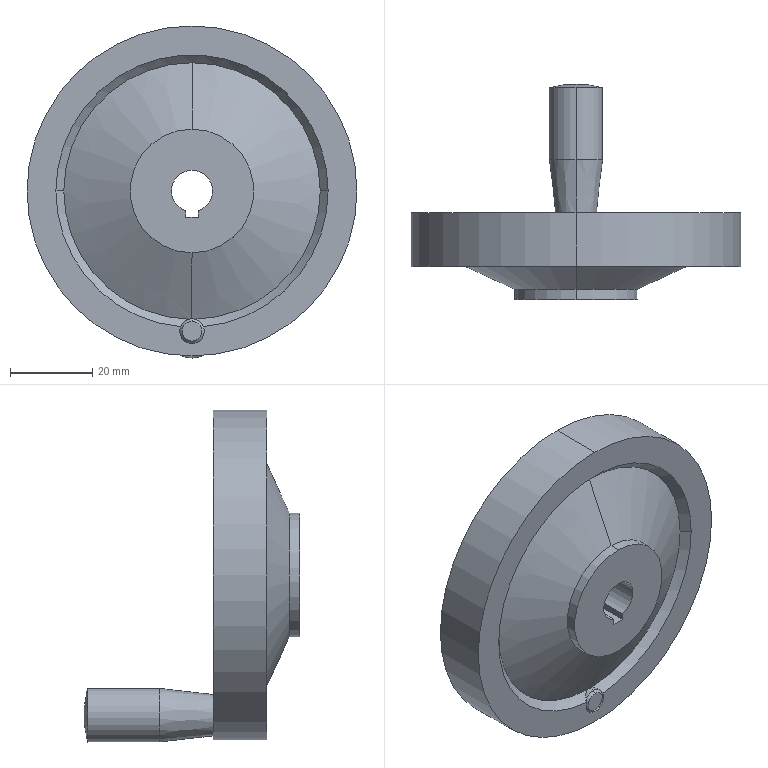Part | SolidWorks | features BaseBody 1 | 1 solid | 35 faces | box 80 x 52.448 x 80.5 mm | volume 63637 mm3 | cylinder 15 | cone 11 | plane 8 | spline 1 | commonest cylinder face diameters 30 x4 6 x3 10 x2 13 x2 56 x2 80 x2
STEP:
#1=CARTESIAN_POINT('',(0.,8.,40.));
#2=VERTEX_POINT('',#1);
#3=CARTESIAN_POINT('',(0.,8.,-40.));
#4=VERTEX_POINT('',#3);
#5=CARTESIAN_POINT('',(0.,8.,0.));
#6=DIRECTION('',(0.,1.,0.));
#7=DIRECTION('',(0.,0.,1.));
#8=AXIS2_PLACEMENT_3D('',#5,#6,#7);
#9=CIRCLE('',#8,40.);
#10=EDGE_CURVE('',#2,#4,#9,.T.);
#11=ORIENTED_EDGE('',*,*,#10,.T.);
#12=CARTESIAN_POINT('',(0.,21.,-40.));
#13=VERTEX_POINT('',#12);
#14=CARTESIAN_POINT('',(0.,-50.,-40.));
#15=DIRECTION('',(0.,1.,0.));
#16=VECTOR('',#15,1000.);
#17=LINE('',#14,#16);
#18=EDGE_CURVE('',#4,#13,#17,.T.);
#19=ORIENTED_EDGE('',*,*,#18,.T.);
#20=CARTESIAN_POINT('',(0.,21.,40.));
#21=VERTEX_POINT('',#20);
#22=CARTESIAN_POINT('',(0.,21.,0.));
#23=DIRECTION('',(0.,-1.,0.));
#24=DIRECTION('',(0.,0.,1.));
#25=AXIS2_PLACEMENT_3D('',#22,#23,#24);
#26=CIRCLE('',#25,40.);
#27=EDGE_CURVE('',#13,#21,#26,.T.);
#28=ORIENTED_EDGE('',*,*,#27,.T.);
#29=CARTESIAN_POINT('',(0.,-50.,40.));
#30=DIRECTION('',(0.,1.,0.));
#31=VECTOR('',#30,1000.);
#32=LINE('',#29,#31);
#33=EDGE_CURVE('',#2,#21,#32,.T.);
#34=ORIENTED_EDGE('',*,*,#33,.F.);
#35=EDGE_LOOP('',(#11,#19,#28,#34));
#36=FACE_OUTER_BOUND('',#35,.T.);
#37=CARTESIAN_POINT('',(0.,-50.,0.));
#38=DIRECTION('',(0.,1.,0.));
#39=DIRECTION('',(0.,0.,1.));
#40=AXIS2_PLACEMENT_3D('',#37,#38,#39);
#41=CYLINDRICAL_SURFACE('',#40,40.);
#42=ADVANCED_FACE('',(#36),#41,.T.);
#43=CARTESIAN_POINT('',(-31.09,9.91,0.));
#44=VERTEX_POINT('',#43);
#45=CARTESIAN_POINT('',(-0.6977,9.91,-31.082));
#46=VERTEX_POINT('',#45);
#47=CARTESIAN_POINT('',(0.,9.91,0.));
#48=DIRECTION('',(0.,-1.,0.));
#49=DIRECTION('',(0.,0.,-1.));
#50=AXIS2_PLACEMENT_3D('',#47,#48,#49);
#51=CIRCLE('',#50,31.09);
#52=EDGE_CURVE('',#44,#46,#51,.T.);
#53=ORIENTED_EDGE('',*,*,#52,.F.);
#54=CARTESIAN_POINT('',(-33.,8.,0.));
#55=VERTEX_POINT('',#54);
#56=CARTESIAN_POINT('',(-33.,8.,0.));
#57=DIRECTION('',(-0.7071,-0.7071,0.));
#58=VECTOR('',#57,1000.);
#59=LINE('',#56,#58);
#60=EDGE_CURVE('',#44,#55,#59,.T.);
#61=ORIENTED_EDGE('',*,*,#60,.T.);
#62=CARTESIAN_POINT('',(-2.784,8.,-32.882));
#63=VERTEX_POINT('',#62);
#64=CARTESIAN_POINT('',(0.,8.,0.));
#65=DIRECTION('',(0.,1.,0.));
#66=DIRECTION('',(1.,0.,0.));
#67=AXIS2_PLACEMENT_3D('',#64,#65,#66);
#68=CIRCLE('',#67,33.);
#69=EDGE_CURVE('',#63,#55,#68,.T.);
#70=ORIENTED_EDGE('',*,*,#69,.F.);
#71=CARTESIAN_POINT('',(-2.5,8.561,-32.342));
#72=VERTEX_POINT('',#71);
#73=CARTESIAN_POINT('',(-2.784,8.,-32.882));
#74=CARTESIAN_POINT('',(-2.709,8.192,-32.696));
#75=CARTESIAN_POINT('',(-2.616,8.379,-32.516));
#76=CARTESIAN_POINT('',(-2.5,8.561,-32.342));
#77=B_SPLINE_CURVE_WITH_KNOTS('',3,(#73,#74,#75,#76),.UNSPECIFIED.,.F.,.F.,(4,4),(0.,0.0008292),.UNSPECIFIED.);
#78=EDGE_CURVE('',#63,#72,#77,.T.);
#79=ORIENTED_EDGE('',*,*,#78,.T.);
#80=CARTESIAN_POINT('',(-0.6977,9.91,-31.082));
#81=CARTESIAN_POINT('',(-0.9084,9.855,-31.133));
#82=CARTESIAN_POINT('',(-1.102,9.778,-31.203));
#83=CARTESIAN_POINT('',(-1.463,9.593,-31.373));
#84=CARTESIAN_POINT('',(-1.63,9.483,-31.475));
#85=CARTESIAN_POINT('',(-2.078,9.129,-31.805));
#86=CARTESIAN_POINT('',(-2.315,8.853,-32.063));
#87=CARTESIAN_POINT('',(-2.5,8.561,-32.342));
#88=B_SPLINE_CURVE_WITH_KNOTS('',3,(#80,#81,#82,#83,#84,#85,#86,#87),.UNSPECIFIED.,.F.,.F.,(4,2,2,4),(0.,0.0006578,0.001316,0.002631),.UNSPECIFIED.);
#89=EDGE_CURVE('',#46,#72,#88,.T.);
#90=ORIENTED_EDGE('',*,*,#89,.F.);
#91=EDGE_LOOP('',(#53,#61,#70,#79,#90));
#92=FACE_OUTER_BOUND('',#91,.T.);
#93=CARTESIAN_POINT('',(0.,8.,0.));
#94=DIRECTION('',(0.,-1.,0.));
#95=DIRECTION('',(1.,0.,0.));
#96=AXIS2_PLACEMENT_3D('',#93,#94,#95);
#97=CONICAL_SURFACE('',#96,33.,0.7854);
#98=ADVANCED_FACE('',(#92),#97,.F.);
#99=ORIENTED_EDGE('',*,*,#60,.F.);
#100=CARTESIAN_POINT('',(0.,9.91,31.09));
#101=VERTEX_POINT('',#100);
#102=CARTESIAN_POINT('',(0.,9.91,0.));
#103=DIRECTION('',(0.,-1.,0.));
#104=DIRECTION('',(0.,0.,-1.));
#105=AXIS2_PLACEMENT_3D('',#102,#103,#104);
#106=CIRCLE('',#105,31.09);
#107=EDGE_CURVE('',#101,#44,#106,.T.);
#108=ORIENTED_EDGE('',*,*,#107,.F.);
#109=CARTESIAN_POINT('',(31.09,9.91,0.));
#110=VERTEX_POINT('',#109);
#111=CARTESIAN_POINT('',(0.,9.91,0.));
#112=DIRECTION('',(0.,-1.,0.));
#113=DIRECTION('',(0.,0.,-1.));
#114=AXIS2_PLACEMENT_3D('',#111,#112,#113);
#115=CIRCLE('',#114,31.09);
#116=EDGE_CURVE('',#110,#101,#115,.T.);
#117=ORIENTED_EDGE('',*,*,#116,.F.);
#118=CARTESIAN_POINT('',(33.,8.,0.));
#119=VERTEX_POINT('',#118);
#120=CARTESIAN_POINT('',(33.,8.,0.));
#121=DIRECTION('',(0.7071,-0.7071,0.));
#122=VECTOR('',#121,1000.);
#123=LINE('',#120,#122);
#124=EDGE_CURVE('',#110,#119,#123,.T.);
#125=ORIENTED_EDGE('',*,*,#124,.T.);
#126=CARTESIAN_POINT('',(0.,8.,0.));
#127=DIRECTION('',(0.,1.,0.));
#128=DIRECTION('',(1.,0.,0.));
#129=AXIS2_PLACEMENT_3D('',#126,#127,#128);
#130=CIRCLE('',#129,33.);
#131=EDGE_CURVE('',#55,#119,#130,.T.);
#132=ORIENTED_EDGE('',*,*,#131,.F.);
#133=EDGE_LOOP('',(#99,#108,#117,#125,#132));
#134=FACE_OUTER_BOUND('',#133,.T.);
#135=CARTESIAN_POINT('',(0.,8.,0.));
#136=DIRECTION('',(0.,-1.,0.));
#137=DIRECTION('',(1.,0.,0.));
#138=AXIS2_PLACEMENT_3D('',#135,#136,#137);
#139=CONICAL_SURFACE('',#138,33.,0.7854);
#140=ADVANCED_FACE('',(#134),#139,.F.);
#141=CARTESIAN_POINT('',(0.,21.,-39.006));
#142=VERTEX_POINT('',#141);
#143=CARTESIAN_POINT('',(0.,21.,-28.994));
#144=VERTEX_POINT('',#143);
#145=CARTESIAN_POINT('',(0.,21.,-34.));
#146=DIRECTION('',(0.,-1.,0.));
#147=DIRECTION('',(0.,0.,1.));
#148=AXIS2_PLACEMENT_3D('',#145,#146,#147);
#149=CIRCLE('',#148,5.006);
#150=EDGE_CURVE('',#142,#144,#149,.T.);
#151=ORIENTED_EDGE('',*,*,#150,.F.);
#152=CARTESIAN_POINT('',(0.,33.948,-40.5));
#153=VERTEX_POINT('',#152);
#154=CARTESIAN_POINT('',(0.,33.948,-40.5));
#155=DIRECTION('',(0.,0.9934,-0.1146));
#156=VECTOR('',#155,1000.);
#157=LINE('',#154,#156);
#158=EDGE_CURVE('',#142,#153,#157,.T.);
#159=ORIENTED_EDGE('',*,*,#158,.T.);
#160=CARTESIAN_POINT('',(0.,33.948,-27.5));
#161=VERTEX_POINT('',#160);
#162=CARTESIAN_POINT('',(0.,33.948,-34.));
#163=DIRECTION('',(0.,-1.,0.));
#164=DIRECTION('',(0.,0.,1.));
#165=AXIS2_PLACEMENT_3D('',#162,#163,#164);
#166=CIRCLE('',#165,6.5);
#167=EDGE_CURVE('',#153,#161,#166,.T.);
#168=ORIENTED_EDGE('',*,*,#167,.T.);
#169=CARTESIAN_POINT('',(0.,33.948,-27.5));
#170=DIRECTION('',(0.,0.9934,0.1146));
#171=VECTOR('',#170,1000.);
#172=LINE('',#169,#171);
#173=EDGE_CURVE('',#144,#161,#172,.T.);
#174=ORIENTED_EDGE('',*,*,#173,.F.);
#175=EDGE_LOOP('',(#151,#159,#168,#174));
#176=FACE_OUTER_BOUND('',#175,.T.);
#177=CARTESIAN_POINT('',(0.,33.948,-34.));
#178=DIRECTION('',(0.,1.,0.));
#179=DIRECTION('',(0.,0.,1.));
#180=AXIS2_PLACEMENT_3D('',#177,#178,#179);
#181=CONICAL_SURFACE('',#180,6.5,0.1149);
#182=ADVANCED_FACE('',(#176),#181,.T.);
#183=CARTESIAN_POINT('',(0.,17.75,-28.));
#184=VERTEX_POINT('',#183);
#185=CARTESIAN_POINT('',(0.,17.75,28.));
#186=VERTEX_POINT('',#185);
#187=CARTESIAN_POINT('',(0.,17.75,0.));
#188=DIRECTION('',(0.,1.,0.));
#189=DIRECTION('',(0.,0.,1.));
#190=AXIS2_PLACEMENT_3D('',#187,#188,#189);
#191=CIRCLE('',#190,28.);
#192=EDGE_CURVE('',#184,#186,#191,.T.);
#193=ORIENTED_EDGE('',*,*,#192,.F.);
#194=CARTESIAN_POINT('',(0.,21.,-28.));
#195=VERTEX_POINT('',#194);
#196=CARTESIAN_POINT('',(0.,-50.,-28.));
#197=DIRECTION('',(0.,1.,0.));
#198=VECTOR('',#197,1000.);
#199=LINE('',#196,#198);
#200=EDGE_CURVE('',#184,#195,#199,.T.);
#201=ORIENTED_EDGE('',*,*,#200,.T.);
#202=CARTESIAN_POINT('',(0.,21.,28.));
#203=VERTEX_POINT('',#202);
#204=CARTESIAN_POINT('',(0.,21.,0.));
#205=DIRECTION('',(0.,-1.,0.));
#206=DIRECTION('',(0.,0.,1.));
#207=AXIS2_PLACEMENT_3D('',#204,#205,#206);
#208=CIRCLE('',#207,28.);
#209=EDGE_CURVE('',#203,#195,#208,.T.);
#210=ORIENTED_EDGE('',*,*,#209,.F.);
#211=CARTESIAN_POINT('',(0.,-50.,28.));
#212=DIRECTION('',(0.,1.,0.));
#213=VECTOR('',#212,1000.);
#214=LINE('',#211,#213);
#215=EDGE_CURVE('',#186,#203,#214,.T.);
#216=ORIENTED_EDGE('',*,*,#215,.F.);
#217=EDGE_LOOP('',(#193,#201,#210,#216));
#218=FACE_OUTER_BOUND('',#217,.T.);
#219=CARTESIAN_POINT('',(0.,-50.,0.));
#220=DIRECTION('',(0.,1.,0.));
#221=DIRECTION('',(0.,0.,1.));
#222=AXIS2_PLACEMENT_3D('',#219,#220,#221);
#223=CYLINDRICAL_SURFACE('',#222,28.);
#224=ADVANCED_FACE('',(#218),#223,.F.);
#225=CARTESIAN_POINT('',(0.,7.948,-31.613));
#226=VERTEX_POINT('',#225);
#227=CARTESIAN_POINT('',(0.,7.948,-36.387));
#228=VERTEX_POINT('',#227);
#229=CARTESIAN_POINT('',(0.,7.948,-34.));
#230=DIRECTION('',(0.,1.,0.));
#231=DIRECTION('',(0.,0.,1.));
#232=AXIS2_PLACEMENT_3D('',#229,#230,#231);
#233=CIRCLE('',#232,2.387);
#234=EDGE_CURVE('',#226,#228,#233,.T.);
#235=ORIENTED_EDGE('',*,*,#234,.T.);
#236=CARTESIAN_POINT('',(0.,8.561,-37.));
#237=VERTEX_POINT('',#236);
#238=CARTESIAN_POINT('',(0.,8.561,-37.));
#239=DIRECTION('',(0.,0.7071,-0.7071));
#240=VECTOR('',#239,1000.);
#241=LINE('',#238,#240);
#242=EDGE_CURVE('',#228,#237,#241,.T.);
#243=ORIENTED_EDGE('',*,*,#242,.T.);
#244=CARTESIAN_POINT('',(2.5,8.561,-32.342));
#245=VERTEX_POINT('',#244);
#246=CARTESIAN_POINT('',(0.,8.561,-34.));
#247=DIRECTION('',(0.,-1.,0.));
#248=DIRECTION('',(0.,0.,1.));
#249=AXIS2_PLACEMENT_3D('',#246,#247,#248);
#250=CIRCLE('',#249,3.);
#251=EDGE_CURVE('',#237,#245,#250,.T.);
#252=ORIENTED_EDGE('',*,*,#251,.T.);
#253=CARTESIAN_POINT('',(0.,8.561,-31.));
#254=VERTEX_POINT('',#253);
#255=CARTESIAN_POINT('',(0.,8.561,-34.));
#256=DIRECTION('',(0.,-1.,0.));
#257=DIRECTION('',(0.,0.,1.));
#258=AXIS2_PLACEMENT_3D('',#255,#256,#257);
#259=CIRCLE('',#258,3.);
#260=EDGE_CURVE('',#245,#254,#259,.T.);
#261=ORIENTED_EDGE('',*,*,#260,.T.);
#262=CARTESIAN_POINT('',(0.,8.561,-31.));
#263=DIRECTION('',(0.,0.7071,0.7071));
#264=VECTOR('',#263,1000.);
#265=LINE('',#262,#264);
#266=EDGE_CURVE('',#226,#254,#265,.T.);
#267=ORIENTED_EDGE('',*,*,#266,.F.);
#268=EDGE_LOOP('',(#235,#243,#252,#261,#267));
#269=FACE_OUTER_BOUND('',#268,.T.);
#270=CARTESIAN_POINT('',(0.,8.561,-34.));
#271=DIRECTION('',(0.,1.,0.));
#272=DIRECTION('',(0.,0.,1.));
#273=AXIS2_PLACEMENT_3D('',#270,#271,#272);
#274=CONICAL_SURFACE('',#273,3.,0.7854);
#275=ADVANCED_FACE('',(#269),#274,.T.);
#276=CARTESIAN_POINT('',(0.,8.561,-34.));
#277=DIRECTION('',(0.,-1.,0.));
#278=DIRECTION('',(0.,0.,1.));
#279=AXIS2_PLACEMENT_3D('',#276,#277,#278);
#280=CIRCLE('',#279,3.);
#281=EDGE_CURVE('',#254,#72,#280,.T.);
#282=ORIENTED_EDGE('',*,*,#281,.F.);
#283=CARTESIAN_POINT('',(0.,9.868,-31.));
#284=VERTEX_POINT('',#283);
#285=CARTESIAN_POINT('',(0.,-50.052,-31.));
#286=DIRECTION('',(0.,1.,0.));
#287=VECTOR('',#286,1000.);
#288=LINE('',#285,#287);
#289=EDGE_CURVE('',#254,#284,#288,.T.);
#290=ORIENTED_EDGE('',*,*,#289,.T.);
#291=CARTESIAN_POINT('',(0.,9.868,-31.));
#292=CARTESIAN_POINT('',(-0.2338,9.868,-31.));
#293=CARTESIAN_POINT('',(-0.4696,9.882,-31.028));
#294=CARTESIAN_POINT('',(-0.6977,9.91,-31.082));
#295=B_SPLINE_CURVE_WITH_KNOTS('',3,(#291,#292,#293,#294),.UNSPECIFIED.,.F.,.F.,(4,4),(0.0007033,0.001401),.UNSPECIFIED.);
#296=EDGE_CURVE('',#284,#46,#295,.T.);
#297=ORIENTED_EDGE('',*,*,#296,.T.);
#298=ORIENTED_EDGE('',*,*,#89,.T.);
#299=EDGE_LOOP('',(#282,#290,#297,#298));
#300=FACE_OUTER_BOUND('',#299,.T.);
#301=CARTESIAN_POINT('',(0.,-50.052,-34.));
#302=DIRECTION('',(0.,1.,0.));
#303=DIRECTION('',(0.,0.,1.));
#304=AXIS2_PLACEMENT_3D('',#301,#302,#303);
#305=CYLINDRICAL_SURFACE('',#304,3.);
#306=ADVANCED_FACE('',(#300),#305,.T.);
#307=CARTESIAN_POINT('',(0.,2.5,15.));
#308=VERTEX_POINT('',#307);
#309=CARTESIAN_POINT('',(0.,2.5,-15.));
#310=VERTEX_POINT('',#309);
#311=CARTESIAN_POINT('',(0.,2.5,0.));
#312=DIRECTION('',(0.,1.,0.));
#313=DIRECTION('',(0.,0.,1.));
#314=AXIS2_PLACEMENT_3D('',#311,#312,#313);
#315=CIRCLE('',#314,15.);
#316=EDGE_CURVE('',#308,#310,#315,.T.);
#317=ORIENTED_EDGE('',*,*,#316,.T.);
#318=CARTESIAN_POINT('',(0.,9.91,-31.09));
#319=DIRECTION('',(0.,0.4183,-0.9083));
#320=VECTOR('',#319,1000.);
#321=LINE('',#318,#320);
#322=EDGE_CURVE('',#310,#284,#321,.T.);
#323=ORIENTED_EDGE('',*,*,#322,.T.);
#324=CARTESIAN_POINT('',(0.6977,9.91,-31.082));
#325=VERTEX_POINT('',#324);
#326=CARTESIAN_POINT('',(0.6977,9.91,-31.082));
#327=CARTESIAN_POINT('',(0.468,9.882,-31.027));
#328=CARTESIAN_POINT('',(0.2354,9.868,-31.));
#329=CARTESIAN_POINT('',(0.,9.868,-31.));
#330=B_SPLINE_CURVE_WITH_KNOTS('',3,(#326,#327,#328,#329),.UNSPECIFIED.,.F.,.F.,(4,4),(0.,0.0007033),.UNSPECIFIED.);
#331=EDGE_CURVE('',#325,#284,#330,.T.);
#332=ORIENTED_EDGE('',*,*,#331,.F.);
#333=CARTESIAN_POINT('',(0.,9.91,0.));
#334=DIRECTION('',(0.,-1.,0.));
#335=DIRECTION('',(0.,0.,-1.));
#336=AXIS2_PLACEMENT_3D('',#333,#334,#335);
#337=CIRCLE('',#336,31.09);
#338=EDGE_CURVE('',#325,#110,#337,.T.);
#339=ORIENTED_EDGE('',*,*,#338,.T.);
#340=ORIENTED_EDGE('',*,*,#116,.T.);
#341=CARTESIAN_POINT('',(0.,9.91,31.09));
#342=DIRECTION('',(0.,0.4183,0.9083));
#343=VECTOR('',#342,1000.);
#344=LINE('',#341,#343);
#345=EDGE_CURVE('',#308,#101,#344,.T.);
#346=ORIENTED_EDGE('',*,*,#345,.F.);
#347=EDGE_LOOP('',(#317,#323,#332,#339,#340,#346));
#348=FACE_OUTER_BOUND('',#347,.T.);
#349=CARTESIAN_POINT('',(0.,9.91,0.));
#350=DIRECTION('',(0.,1.,0.));
#351=DIRECTION('',(0.,0.,1.));
#352=AXIS2_PLACEMENT_3D('',#349,#350,#351);
#353=CONICAL_SURFACE('',#352,31.09,1.139);
#354=ADVANCED_FACE('',(#348),#353,.T.);
#355=ORIENTED_EDGE('',*,*,#167,.F.);
#356=CARTESIAN_POINT('',(0.,51.448,-40.5));
#357=VERTEX_POINT('',#356);
#358=CARTESIAN_POINT('',(0.,-50.052,-40.5));
#359=DIRECTION('',(0.,1.,0.));
#360=VECTOR('',#359,1000.);
#361=LINE('',#358,#360);
#362=EDGE_CURVE('',#153,#357,#361,.T.);
#363=ORIENTED_EDGE('',*,*,#362,.T.);
#364=CARTESIAN_POINT('',(0.,51.448,-27.5));
#365=VERTEX_POINT('',#364);
#366=CARTESIAN_POINT('',(0.,51.448,-34.));
#367=DIRECTION('',(0.,-1.,0.));
#368=DIRECTION('',(0.,0.,1.));
#369=AXIS2_PLACEMENT_3D('',#366,#367,#368);
#370=CIRCLE('',#369,6.5);
#371=EDGE_CURVE('',#357,#365,#370,.T.);
#372=ORIENTED_EDGE('',*,*,#371,.T.);
#373=CARTESIAN_POINT('',(0.,-50.052,-27.5));
#374=DIRECTION('',(0.,1.,0.));
#375=VECTOR('',#374,1000.);
#376=LINE('',#373,#375);
#377=EDGE_CURVE('',#161,#365,#376,.T.);
#378=ORIENTED_EDGE('',*,*,#377,.F.);
#379=EDGE_LOOP('',(#355,#363,#372,#378));
#380=FACE_OUTER_BOUND('',#379,.T.);
#381=CARTESIAN_POINT('',(0.,-50.052,-34.));
#382=DIRECTION('',(0.,1.,0.));
#383=DIRECTION('',(0.,0.,1.));
#384=AXIS2_PLACEMENT_3D('',#381,#382,#383);
#385=CYLINDRICAL_SURFACE('',#384,6.5);
#386=ADVANCED_FACE('',(#380),#385,.T.);
#387=CARTESIAN_POINT('',(0.,13.5,-15.));
#388=VERTEX_POINT('',#387);
#389=CARTESIAN_POINT('',(0.,13.5,15.));
#390=VERTEX_POINT('',#389);
#391=CARTESIAN_POINT('',(0.,13.5,0.));
#392=DIRECTION('',(0.,1.,0.));
#393=DIRECTION('',(0.,0.,1.));
#394=AXIS2_PLACEMENT_3D('',#391,#392,#393);
#395=CIRCLE('',#394,15.);
#396=EDGE_CURVE('',#388,#390,#395,.T.);
#397=ORIENTED_EDGE('',*,*,#396,.F.);
#398=CARTESIAN_POINT('',(0.,17.75,-28.));
#399=DIRECTION('',(0.,0.3107,-0.9505));
#400=VECTOR('',#399,1000.);
#401=LINE('',#398,#400);
#402=EDGE_CURVE('',#388,#184,#401,.T.);
#403=ORIENTED_EDGE('',*,*,#402,.T.);
#404=ORIENTED_EDGE('',*,*,#192,.T.);
#405=CARTESIAN_POINT('',(0.,17.75,28.));
#406=DIRECTION('',(0.,0.3107,0.9505));
#407=VECTOR('',#406,1000.);
#408=LINE('',#405,#407);
#409=EDGE_CURVE('',#390,#186,#408,.T.);
#410=ORIENTED_EDGE('',*,*,#409,.F.);
#411=EDGE_LOOP('',(#397,#403,#404,#410));
#412=FACE_OUTER_BOUND('',#411,.T.);
#413=CARTESIAN_POINT('',(0.,17.75,0.));
#414=DIRECTION('',(0.,1.,0.));
#415=DIRECTION('',(0.,0.,1.));
#416=AXIS2_PLACEMENT_3D('',#413,#414,#415);
#417=CONICAL_SURFACE('',#416,28.,1.255);
#418=ADVANCED_FACE('',(#412),#417,.F.);
#419=CARTESIAN_POINT('',(0.,0.,15.));
#420=VERTEX_POINT('',#419);
#421=CARTESIAN_POINT('',(0.,0.,-15.));
#422=VERTEX_POINT('',#421);
#423=CARTESIAN_POINT('',(0.,0.,0.));
#424=DIRECTION('',(0.,1.,0.));
#425=DIRECTION('',(0.,0.,1.));
#426=AXIS2_PLACEMENT_3D('',#423,#424,#425);
#427=CIRCLE('',#426,15.);
#428=EDGE_CURVE('',#420,#422,#427,.T.);
#429=ORIENTED_EDGE('',*,*,#428,.T.);
#430=CARTESIAN_POINT('',(0.,-50.,-15.));
#431=DIRECTION('',(0.,1.,0.));
#432=VECTOR('',#431,1000.);
#433=LINE('',#430,#432);
#434=EDGE_CURVE('',#422,#310,#433,.T.);
#435=ORIENTED_EDGE('',*,*,#434,.T.);
#436=ORIENTED_EDGE('',*,*,#316,.F.);
#437=CARTESIAN_POINT('',(0.,-50.,15.));
#438=DIRECTION('',(0.,1.,0.));
#439=VECTOR('',#438,1000.);
#440=LINE('',#437,#439);
#441=EDGE_CURVE('',#420,#308,#440,.T.);
#442=ORIENTED_EDGE('',*,*,#441,.F.);
#443=EDGE_LOOP('',(#429,#435,#436,#442));
#444=FACE_OUTER_BOUND('',#443,.T.);
#445=CARTESIAN_POINT('',(0.,-50.,0.));
#446=DIRECTION('',(0.,1.,0.));
#447=DIRECTION('',(0.,0.,1.));
#448=AXIS2_PLACEMENT_3D('',#445,#446,#447);
#449=CYLINDRICAL_SURFACE('',#448,15.);
#450=ADVANCED_FACE('',(#444),#449,.T.);
#451=CARTESIAN_POINT('',(0.,13.5,0.));
#452=DIRECTION('',(0.,1.,0.));
#453=DIRECTION('',(0.,0.,1.));
#454=AXIS2_PLACEMENT_3D('',#451,#452,#453);
#455=CIRCLE('',#454,15.);
#456=EDGE_CURVE('',#390,#388,#455,.T.);
#457=ORIENTED_EDGE('',*,*,#456,.T.);
#458=CARTESIAN_POINT('',(0.,16.,-15.));
#459=VERTEX_POINT('',#458);
#460=CARTESIAN_POINT('',(0.,-50.,-15.));
#461=DIRECTION('',(0.,1.,0.));
#462=VECTOR('',#461,1000.);
#463=LINE('',#460,#462);
#464=EDGE_CURVE('',#388,#459,#463,.T.);
#465=ORIENTED_EDGE('',*,*,#464,.T.);
#466=CARTESIAN_POINT('',(0.,16.,15.));
#467=VERTEX_POINT('',#466);
#468=CARTESIAN_POINT('',(0.,16.,0.));
#469=DIRECTION('',(0.,-1.,0.));
#470=DIRECTION('',(0.,0.,1.));
#471=AXIS2_PLACEMENT_3D('',#468,#469,#470);
#472=CIRCLE('',#471,15.);
#473=EDGE_CURVE('',#459,#467,#472,.T.);
#474=ORIENTED_EDGE('',*,*,#473,.T.);
#475=CARTESIAN_POINT('',(0.,-50.,15.));
#476=DIRECTION('',(0.,1.,0.));
#477=VECTOR('',#476,1000.);
#478=LINE('',#475,#477);
#479=EDGE_CURVE('',#390,#467,#478,.T.);
#480=ORIENTED_EDGE('',*,*,#479,.F.);
#481=EDGE_LOOP('',(#457,#465,#474,#480));
#482=FACE_OUTER_BOUND('',#481,.T.);
#483=CARTESIAN_POINT('',(0.,-50.,0.));
#484=DIRECTION('',(0.,1.,0.));
#485=DIRECTION('',(0.,0.,1.));
#486=AXIS2_PLACEMENT_3D('',#483,#484,#485);
#487=CYLINDRICAL_SURFACE('',#486,15.);
#488=ADVANCED_FACE('',(#482),#487,.T.);
#489=CARTESIAN_POINT('',(0.,0.,5.));
#490=VERTEX_POINT('',#489);
#491=CARTESIAN_POINT('',(1.5,0.,-4.77));
#492=VERTEX_POINT('',#491);
#493=CARTESIAN_POINT('',(0.,0.,0.));
#494=DIRECTION('',(0.,1.,0.));
#495=DIRECTION('',(0.,0.,1.));
#496=AXIS2_PLACEMENT_3D('',#493,#494,#495);
#497=CIRCLE('',#496,5.);
#498=EDGE_CURVE('',#490,#492,#497,.T.);
#499=ORIENTED_EDGE('',*,*,#498,.F.);
#500=CARTESIAN_POINT('',(0.,16.,5.));
#501=VERTEX_POINT('',#500);
#502=CARTESIAN_POINT('',(0.,-50.,5.));
#503=DIRECTION('',(0.,1.,0.));
#504=VECTOR('',#503,1000.);
#505=LINE('',#502,#504);
#506=EDGE_CURVE('',#490,#501,#505,.T.);
#507=ORIENTED_EDGE('',*,*,#506,.T.);
#508=CARTESIAN_POINT('',(1.5,16.,-4.77));
#509=VERTEX_POINT('',#508);
#510=CARTESIAN_POINT('',(0.,16.,0.));
#511=DIRECTION('',(0.,-1.,0.));
#512=DIRECTION('',(0.,0.,1.));
#513=AXIS2_PLACEMENT_3D('',#510,#511,#512);
#514=CIRCLE('',#513,5.);
#515=EDGE_CURVE('',#509,#501,#514,.T.);
#516=ORIENTED_EDGE('',*,*,#515,.F.);
#517=CARTESIAN_POINT('',(1.5,-50.,-4.77));
#518=DIRECTION('',(0.,1.,0.));
#519=VECTOR('',#518,1000.);
#520=LINE('',#517,#519);
#521=EDGE_CURVE('',#492,#509,#520,.T.);
#522=ORIENTED_EDGE('',*,*,#521,.F.);
#523=EDGE_LOOP('',(#499,#507,#516,#522));
#524=FACE_OUTER_BOUND('',#523,.T.);
#525=CARTESIAN_POINT('',(0.,-50.,0.));
#526=DIRECTION('',(0.,1.,0.));
#527=DIRECTION('',(0.,0.,1.));
#528=AXIS2_PLACEMENT_3D('',#525,#526,#527);
#529=CYLINDRICAL_SURFACE('',#528,5.);
#530=ADVANCED_FACE('',(#524),#529,.F.);
#531=ORIENTED_EDGE('',*,*,#18,.F.);
#532=CARTESIAN_POINT('',(0.,8.,0.));
#533=DIRECTION('',(0.,1.,0.));
#534=DIRECTION('',(0.,0.,1.));
#535=AXIS2_PLACEMENT_3D('',#532,#533,#534);
#536=CIRCLE('',#535,40.);
#537=EDGE_CURVE('',#4,#2,#536,.T.);
#538=ORIENTED_EDGE('',*,*,#537,.T.);
#539=ORIENTED_EDGE('',*,*,#33,.T.);
#540=CARTESIAN_POINT('',(0.,21.,0.));
#541=DIRECTION('',(0.,-1.,0.));
#542=DIRECTION('',(0.,0.,1.));
#543=AXIS2_PLACEMENT_3D('',#540,#541,#542);
#544=CIRCLE('',#543,40.);
#545=EDGE_CURVE('',#21,#13,#544,.T.);
#546=ORIENTED_EDGE('',*,*,#545,.T.);
#547=EDGE_LOOP('',(#531,#538,#539,#546));
#548=FACE_OUTER_BOUND('',#547,.T.);
#549=CARTESIAN_POINT('',(0.,-50.,0.));
#550=DIRECTION('',(0.,1.,0.));
#551=DIRECTION('',(0.,0.,1.));
#552=AXIS2_PLACEMENT_3D('',#549,#550,#551);
#553=CYLINDRICAL_SURFACE('',#552,40.);
#554=ADVANCED_FACE('',(#548),#553,.T.);
#555=ORIENTED_EDGE('',*,*,#69,.T.);
#556=ORIENTED_EDGE('',*,*,#131,.T.);
#557=CARTESIAN_POINT('',(2.784,8.,-32.882));
#558=VERTEX_POINT('',#557);
#559=CARTESIAN_POINT('',(0.,8.,0.));
#560=DIRECTION('',(0.,1.,0.));
#561=DIRECTION('',(1.,0.,0.));
#562=AXIS2_PLACEMENT_3D('',#559,#560,#561);
#563=CIRCLE('',#562,33.);
#564=EDGE_CURVE('',#119,#558,#563,.T.);
#565=ORIENTED_EDGE('',*,*,#564,.T.);
#566=CARTESIAN_POINT('',(0.,8.,-34.));
#567=DIRECTION('',(0.,1.,0.));
#568=DIRECTION('',(0.,0.,1.));
#569=AXIS2_PLACEMENT_3D('',#566,#567,#568);
#570=CIRCLE('',#569,3.);
#571=EDGE_CURVE('',#558,#63,#570,.T.);
#572=ORIENTED_EDGE('',*,*,#571,.T.);
#573=EDGE_LOOP('',(#555,#556,#565,#572));
#574=FACE_BOUND('',#573,.T.);
#575=ORIENTED_EDGE('',*,*,#10,.F.);
#576=ORIENTED_EDGE('',*,*,#537,.F.);
#577=EDGE_LOOP('',(#575,#576));
#578=FACE_OUTER_BOUND('',#577,.T.);
#579=CARTESIAN_POINT('',(0.,8.,33.));
#580=DIRECTION('',(0.,-1.,0.));
#581=DIRECTION('',(0.,0.,-1.));
#582=AXIS2_PLACEMENT_3D('',#579,#580,#581);
#583=PLANE('',#582);
#584=ADVANCED_FACE('',(#574,#578),#583,.T.);
#585=ORIENTED_EDGE('',*,*,#545,.F.);
#586=ORIENTED_EDGE('',*,*,#27,.F.);
#587=EDGE_LOOP('',(#585,#586));
#588=FACE_OUTER_BOUND('',#587,.T.);
#589=CARTESIAN_POINT('',(0.,21.,-34.));
#590=DIRECTION('',(0.,-1.,0.));
#591=DIRECTION('',(0.,0.,1.));
#592=AXIS2_PLACEMENT_3D('',#589,#590,#591);
#593=CIRCLE('',#592,5.006);
#594=EDGE_CURVE('',#144,#142,#593,.T.);
#595=ORIENTED_EDGE('',*,*,#594,.T.);
#596=ORIENTED_EDGE('',*,*,#150,.T.);
#597=EDGE_LOOP('',(#595,#596));
#598=FACE_BOUND('',#597,.T.);
#599=ORIENTED_EDGE('',*,*,#209,.T.);
#600=CARTESIAN_POINT('',(0.,21.,0.));
#601=DIRECTION('',(0.,-1.,0.));
#602=DIRECTION('',(0.,0.,1.));
#603=AXIS2_PLACEMENT_3D('',#600,#601,#602);
#604=CIRCLE('',#603,28.);
#605=EDGE_CURVE('',#195,#203,#604,.T.);
#606=ORIENTED_EDGE('',*,*,#605,.T.);
#607=EDGE_LOOP('',(#599,#606));
#608=FACE_BOUND('',#607,.T.);
#609=CARTESIAN_POINT('',(0.,21.,40.));
#610=DIRECTION('',(0.,1.,0.));
#611=DIRECTION('',(0.,0.,1.));
#612=AXIS2_PLACEMENT_3D('',#609,#610,#611);
#613=PLANE('',#612);
#614=ADVANCED_FACE('',(#588,#598,#608),#613,.T.);
#615=CARTESIAN_POINT('',(2.5,8.561,-32.342));
#616=CARTESIAN_POINT('',(2.616,8.379,-32.516));
#617=CARTESIAN_POINT('',(2.709,8.192,-32.696));
#618=CARTESIAN_POINT('',(2.784,8.,-32.882));
#619=B_SPLINE_CURVE_WITH_KNOTS('',3,(#615,#616,#617,#618),.UNSPECIFIED.,.F.,.F.,(4,4),(0.,0.0008292),.UNSPECIFIED.);
#620=EDGE_CURVE('',#245,#558,#619,.T.);
#621=ORIENTED_EDGE('',*,*,#620,.F.);
#622=ORIENTED_EDGE('',*,*,#251,.F.);
#623=CARTESIAN_POINT('',(0.,8.561,-34.));
#624=DIRECTION('',(0.,-1.,0.));
#625=DIRECTION('',(0.,0.,1.));
#626=AXIS2_PLACEMENT_3D('',#623,#624,#625);
#627=CIRCLE('',#626,3.);
#628=EDGE_CURVE('',#72,#237,#627,.T.);
#629=ORIENTED_EDGE('',*,*,#628,.F.);
#630=ORIENTED_EDGE('',*,*,#78,.F.);
#631=ORIENTED_EDGE('',*,*,#571,.F.);
#632=EDGE_LOOP('',(#621,#622,#629,#630,#631));
#633=FACE_OUTER_BOUND('',#632,.T.);
#634=CARTESIAN_POINT('',(0.,8.,-34.));
#635=DIRECTION('',(0.,1.,0.));
#636=DIRECTION('',(0.,0.,1.));
#637=AXIS2_PLACEMENT_3D('',#634,#635,#636);
#638=CYLINDRICAL_SURFACE('',#637,3.);
#639=ADVANCED_FACE('',(#633),#638,.F.);
#640=ORIENTED_EDGE('',*,*,#124,.F.);
#641=ORIENTED_EDGE('',*,*,#338,.F.);
#642=CARTESIAN_POINT('',(2.5,8.561,-32.342));
#643=CARTESIAN_POINT('',(2.315,8.853,-32.063));
#644=CARTESIAN_POINT('',(2.083,9.124,-31.809));
#645=CARTESIAN_POINT('',(1.635,9.48,-31.478));
#646=CARTESIAN_POINT('',(1.468,9.59,-31.376));
#647=CARTESIAN_POINT('',(1.106,9.777,-31.204));
#648=CARTESIAN_POINT('',(0.9086,9.855,-31.133));
#649=CARTESIAN_POINT('',(0.6977,9.91,-31.082));
#650=B_SPLINE_CURVE_WITH_KNOTS('',3,(#642,#643,#644,#645,#646,#647,#648,#649),.UNSPECIFIED.,.F.,.F.,(4,2,2,4),(0.,0.001311,0.001967,0.002623),.UNSPECIFIED.);
#651=EDGE_CURVE('',#245,#325,#650,.T.);
#652=ORIENTED_EDGE('',*,*,#651,.F.);
#653=ORIENTED_EDGE('',*,*,#620,.T.);
#654=ORIENTED_EDGE('',*,*,#564,.F.);
#655=EDGE_LOOP('',(#640,#641,#652,#653,#654));
#656=FACE_OUTER_BOUND('',#655,.T.);
#657=CARTESIAN_POINT('',(0.,8.,0.));
#658=DIRECTION('',(0.,-1.,0.));
#659=DIRECTION('',(1.,0.,0.));
#660=AXIS2_PLACEMENT_3D('',#657,#658,#659);
#661=CONICAL_SURFACE('',#660,33.,0.7854);
#662=ADVANCED_FACE('',(#656),#661,.F.);
#663=ORIENTED_EDGE('',*,*,#158,.F.);
#664=ORIENTED_EDGE('',*,*,#594,.F.);
#665=ORIENTED_EDGE('',*,*,#173,.T.);
#666=CARTESIAN_POINT('',(0.,33.948,-34.));
#667=DIRECTION('',(0.,-1.,0.));
#668=DIRECTION('',(0.,0.,1.));
#669=AXIS2_PLACEMENT_3D('',#666,#667,#668);
#670=CIRCLE('',#669,6.5);
#671=EDGE_CURVE('',#161,#153,#670,.T.);
#672=ORIENTED_EDGE('',*,*,#671,.T.);
#673=EDGE_LOOP('',(#663,#664,#665,#672));
#674=FACE_OUTER_BOUND('',#673,.T.);
#675=CARTESIAN_POINT('',(0.,33.948,-34.));
#676=DIRECTION('',(0.,1.,0.));
#677=DIRECTION('',(0.,0.,1.));
#678=AXIS2_PLACEMENT_3D('',#675,#676,#677);
#679=CONICAL_SURFACE('',#678,6.5,0.1149);
#680=ADVANCED_FACE('',(#674),#679,.T.);
#681=ORIENTED_EDGE('',*,*,#200,.F.);
#682=CARTESIAN_POINT('',(0.,17.75,0.));
#683=DIRECTION('',(0.,1.,0.));
#684=DIRECTION('',(0.,0.,1.));
#685=AXIS2_PLACEMENT_3D('',#682,#683,#684);
#686=CIRCLE('',#685,28.);
#687=EDGE_CURVE('',#186,#184,#686,.T.);
#688=ORIENTED_EDGE('',*,*,#687,.F.);
#689=ORIENTED_EDGE('',*,*,#215,.T.);
#690=ORIENTED_EDGE('',*,*,#605,.F.);
#691=EDGE_LOOP('',(#681,#688,#689,#690));
#692=FACE_OUTER_BOUND('',#691,.T.);
#693=CARTESIAN_POINT('',(0.,-50.,0.));
#694=DIRECTION('',(0.,1.,0.));
#695=DIRECTION('',(0.,0.,1.));
#696=AXIS2_PLACEMENT_3D('',#693,#694,#695);
#697=CYLINDRICAL_SURFACE('',#696,28.);
#698=ADVANCED_FACE('',(#692),#697,.F.);
#699=ORIENTED_EDGE('',*,*,#242,.F.);
#700=CARTESIAN_POINT('',(0.,7.948,-34.));
#701=DIRECTION('',(0.,1.,0.));
#702=DIRECTION('',(0.,0.,1.));
#703=AXIS2_PLACEMENT_3D('',#700,#701,#702);
#704=CIRCLE('',#703,2.387);
#705=EDGE_CURVE('',#228,#226,#704,.T.);
#706=ORIENTED_EDGE('',*,*,#705,.T.);
#707=ORIENTED_EDGE('',*,*,#266,.T.);
#708=ORIENTED_EDGE('',*,*,#281,.T.);
#709=ORIENTED_EDGE('',*,*,#628,.T.);
#710=EDGE_LOOP('',(#699,#706,#707,#708,#709));
#711=FACE_OUTER_BOUND('',#710,.T.);
#712=CARTESIAN_POINT('',(0.,8.561,-34.));
#713=DIRECTION('',(0.,1.,0.));
#714=DIRECTION('',(0.,0.,1.));
#715=AXIS2_PLACEMENT_3D('',#712,#713,#714);
#716=CONICAL_SURFACE('',#715,3.,0.7854);
#717=ADVANCED_FACE('',(#711),#716,.T.);
#718=ORIENTED_EDGE('',*,*,#289,.F.);
#719=ORIENTED_EDGE('',*,*,#260,.F.);
#720=ORIENTED_EDGE('',*,*,#651,.T.);
#721=ORIENTED_EDGE('',*,*,#331,.T.);
#722=EDGE_LOOP('',(#718,#719,#720,#721));
#723=FACE_OUTER_BOUND('',#722,.T.);
#724=CARTESIAN_POINT('',(0.,-50.052,-34.));
#725=DIRECTION('',(0.,1.,0.));
#726=DIRECTION('',(0.,0.,1.));
#727=AXIS2_PLACEMENT_3D('',#724,#725,#726);
#728=CYLINDRICAL_SURFACE('',#727,3.);
#729=ADVANCED_FACE('',(#723),#728,.T.);
#730=ORIENTED_EDGE('',*,*,#322,.F.);
#731=CARTESIAN_POINT('',(0.,2.5,0.));
#732=DIRECTION('',(0.,1.,0.));
#733=DIRECTION('',(0.,0.,1.));
#734=AXIS2_PLACEMENT_3D('',#731,#732,#733);
#735=CIRCLE('',#734,15.);
#736=EDGE_CURVE('',#310,#308,#735,.T.);
#737=ORIENTED_EDGE('',*,*,#736,.T.);
#738=ORIENTED_EDGE('',*,*,#345,.T.);
#739=ORIENTED_EDGE('',*,*,#107,.T.);
#740=ORIENTED_EDGE('',*,*,#52,.T.);
#741=ORIENTED_EDGE('',*,*,#296,.F.);
#742=EDGE_LOOP('',(#730,#737,#738,#739,#740,#741));
#743=FACE_OUTER_BOUND('',#742,.T.);
#744=CARTESIAN_POINT('',(0.,9.91,0.));
#745=DIRECTION('',(0.,1.,0.));
#746=DIRECTION('',(0.,0.,1.));
#747=AXIS2_PLACEMENT_3D('',#744,#745,#746);
#748=CONICAL_SURFACE('',#747,31.09,1.139);
#749=ADVANCED_FACE('',(#743),#748,.T.);
#750=ORIENTED_EDGE('',*,*,#362,.F.);
#751=ORIENTED_EDGE('',*,*,#671,.F.);
#752=ORIENTED_EDGE('',*,*,#377,.T.);
#753=CARTESIAN_POINT('',(0.,51.448,-34.));
#754=DIRECTION('',(0.,-1.,0.));
#755=DIRECTION('',(0.,0.,1.));
#756=AXIS2_PLACEMENT_3D('',#753,#754,#755);
#757=CIRCLE('',#756,6.5);
#758=EDGE_CURVE('',#365,#357,#757,.T.);
#759=ORIENTED_EDGE('',*,*,#758,.T.);
#760=EDGE_LOOP('',(#750,#751,#752,#759));
#761=FACE_OUTER_BOUND('',#760,.T.);
#762=CARTESIAN_POINT('',(0.,-50.052,-34.));
#763=DIRECTION('',(0.,1.,0.));
#764=DIRECTION('',(0.,0.,1.));
#765=AXIS2_PLACEMENT_3D('',#762,#763,#764);
#766=CYLINDRICAL_SURFACE('',#765,6.5);
#767=ADVANCED_FACE('',(#761),#766,.T.);
#768=ORIENTED_EDGE('',*,*,#402,.F.);
#769=ORIENTED_EDGE('',*,*,#456,.F.);
#770=ORIENTED_EDGE('',*,*,#409,.T.);
#771=ORIENTED_EDGE('',*,*,#687,.T.);
#772=EDGE_LOOP('',(#768,#769,#770,#771));
#773=FACE_OUTER_BOUND('',#772,.T.);
#774=CARTESIAN_POINT('',(0.,17.75,0.));
#775=DIRECTION('',(0.,1.,0.));
#776=DIRECTION('',(0.,0.,1.));
#777=AXIS2_PLACEMENT_3D('',#774,#775,#776);
#778=CONICAL_SURFACE('',#777,28.,1.255);
#779=ADVANCED_FACE('',(#773),#778,.F.);
#780=ORIENTED_EDGE('',*,*,#234,.F.);
#781=ORIENTED_EDGE('',*,*,#705,.F.);
#782=EDGE_LOOP('',(#780,#781));
#783=FACE_OUTER_BOUND('',#782,.T.);
#784=CARTESIAN_POINT('',(0.,7.948,-36.387));
#785=DIRECTION('',(0.,1.,0.));
#786=DIRECTION('',(0.,0.,1.));
#787=AXIS2_PLACEMENT_3D('',#784,#785,#786);
#788=PLANE('',#787);
#789=ADVANCED_FACE('',(#783),#788,.F.);
#790=ORIENTED_EDGE('',*,*,#434,.F.);
#791=CARTESIAN_POINT('',(0.,0.,0.));
#792=DIRECTION('',(0.,1.,0.));
#793=DIRECTION('',(0.,0.,1.));
#794=AXIS2_PLACEMENT_3D('',#791,#792,#793);
#795=CIRCLE('',#794,15.);
#796=EDGE_CURVE('',#422,#420,#795,.T.);
#797=ORIENTED_EDGE('',*,*,#796,.T.);
#798=ORIENTED_EDGE('',*,*,#441,.T.);
#799=ORIENTED_EDGE('',*,*,#736,.F.);
#800=EDGE_LOOP('',(#790,#797,#798,#799));
#801=FACE_OUTER_BOUND('',#800,.T.);
#802=CARTESIAN_POINT('',(0.,-50.,0.));
#803=DIRECTION('',(0.,1.,0.));
#804=DIRECTION('',(0.,0.,1.));
#805=AXIS2_PLACEMENT_3D('',#802,#803,#804);
#806=CYLINDRICAL_SURFACE('',#805,15.);
#807=ADVANCED_FACE('',(#801),#806,.T.);
#808=ORIENTED_EDGE('',*,*,#758,.F.);
#809=ORIENTED_EDGE('',*,*,#371,.F.);
#810=EDGE_LOOP('',(#808,#809));
#811=FACE_OUTER_BOUND('',#810,.T.);
#812=CARTESIAN_POINT('',(-6.28,50.43,-40.615));
#813=CARTESIAN_POINT('',(-2.154,51.752,-40.615));
#814=CARTESIAN_POINT('',(2.179,51.749,-40.615));
#815=CARTESIAN_POINT('',(6.304,50.422,-40.615));
#816=CARTESIAN_POINT('',(-6.704,51.753,-36.291));
#817=CARTESIAN_POINT('',(-2.299,53.164,-36.291));
#818=CARTESIAN_POINT('',(2.327,53.161,-36.291));
#819=CARTESIAN_POINT('',(6.73,51.745,-36.291));
#820=CARTESIAN_POINT('',(-6.705,51.757,-31.75));
#821=CARTESIAN_POINT('',(-2.299,53.168,-31.75));
#822=CARTESIAN_POINT('',(2.327,53.165,-31.75));
#823=CARTESIAN_POINT('',(6.731,51.749,-31.75));
#824=CARTESIAN_POINT('',(-6.284,50.442,-27.424));
#825=CARTESIAN_POINT('',(-2.155,51.765,-27.424));
#826=CARTESIAN_POINT('',(2.181,51.762,-27.424));
#827=CARTESIAN_POINT('',(6.308,50.434,-27.424));
#828=(BOUNDED_SURFACE()B_SPLINE_SURFACE(3,3,((#812,#813,#814,#815),(#816,#817,#818,#819),(#820,#821,#822,#823),(#824,#825,#826,#827)),.UNSPECIFIED.,.F.,.F.,.F.)B_SPLINE_SURFACE_WITH_KNOTS((4,4),(4,4),(0.,1.),(0.,1.),.UNSPECIFIED.)GEOMETRIC_REPRESENTATION_ITEM()RATIONAL_B_SPLINE_SURFACE(((1.,0.9681,0.9681,1.),(0.9682,0.9374,0.9374,0.9682),(0.9682,0.9374,0.9374,0.9682),(1.,0.9681,0.9681,1.)))REPRESENTATION_ITEM('')SURFACE());
#829=ADVANCED_FACE('',(#811),#828,.T.);
#830=ORIENTED_EDGE('',*,*,#464,.F.);
#831=ORIENTED_EDGE('',*,*,#396,.T.);
#832=ORIENTED_EDGE('',*,*,#479,.T.);
#833=CARTESIAN_POINT('',(0.,16.,0.));
#834=DIRECTION('',(0.,-1.,0.));
#835=DIRECTION('',(0.,0.,1.));
#836=AXIS2_PLACEMENT_3D('',#833,#834,#835);
#837=CIRCLE('',#836,15.);
#838=EDGE_CURVE('',#467,#459,#837,.T.);
#839=ORIENTED_EDGE('',*,*,#838,.T.);
#840=EDGE_LOOP('',(#830,#831,#832,#839));
#841=FACE_OUTER_BOUND('',#840,.T.);
#842=CARTESIAN_POINT('',(0.,-50.,0.));
#843=DIRECTION('',(0.,1.,0.));
#844=DIRECTION('',(0.,0.,1.));
#845=AXIS2_PLACEMENT_3D('',#842,#843,#844);
#846=CYLINDRICAL_SURFACE('',#845,15.);
#847=ADVANCED_FACE('',(#841),#846,.T.);
#848=CARTESIAN_POINT('',(1.5,0.,-6.4));
#849=VERTEX_POINT('',#848);
#850=CARTESIAN_POINT('',(-1.5,0.,-6.4));
#851=VERTEX_POINT('',#850);
#852=CARTESIAN_POINT('',(0.,0.,-6.4));
#853=DIRECTION('',(-1.,0.,0.));
#854=VECTOR('',#853,1000.);
#855=LINE('',#852,#854);
#856=EDGE_CURVE('',#849,#851,#855,.T.);
#857=ORIENTED_EDGE('',*,*,#856,.T.);
#858=CARTESIAN_POINT('',(-1.5,0.,-4.77));
#859=VERTEX_POINT('',#858);
#860=CARTESIAN_POINT('',(-1.5,0.,-6.4));
#861=DIRECTION('',(0.,0.,-1.));
#862=VECTOR('',#861,1000.);
#863=LINE('',#860,#862);
#864=EDGE_CURVE('',#859,#851,#863,.T.);
#865=ORIENTED_EDGE('',*,*,#864,.F.);
#866=CARTESIAN_POINT('',(0.,0.,0.));
#867=DIRECTION('',(0.,1.,0.));
#868=DIRECTION('',(0.,0.,1.));
#869=AXIS2_PLACEMENT_3D('',#866,#867,#868);
#870=CIRCLE('',#869,5.);
#871=EDGE_CURVE('',#859,#490,#870,.T.);
#872=ORIENTED_EDGE('',*,*,#871,.T.);
#873=ORIENTED_EDGE('',*,*,#498,.T.);
#874=CARTESIAN_POINT('',(1.5,0.,0.));
#875=DIRECTION('',(0.,0.,1.));
#876=VECTOR('',#875,1000.);
#877=LINE('',#874,#876);
#878=EDGE_CURVE('',#849,#492,#877,.T.);
#879=ORIENTED_EDGE('',*,*,#878,.F.);
#880=EDGE_LOOP('',(#857,#865,#872,#873,#879));
#881=FACE_BOUND('',#880,.T.);
#882=ORIENTED_EDGE('',*,*,#428,.F.);
#883=ORIENTED_EDGE('',*,*,#796,.F.);
#884=EDGE_LOOP('',(#882,#883));
#885=FACE_OUTER_BOUND('',#884,.T.);
#886=CARTESIAN_POINT('',(0.,0.,5.));
#887=DIRECTION('',(0.,-1.,0.));
#888=DIRECTION('',(0.,0.,-1.));
#889=AXIS2_PLACEMENT_3D('',#886,#887,#888);
#890=PLANE('',#889);
#891=ADVANCED_FACE('',(#881,#885),#890,.T.);
#892=ORIENTED_EDGE('',*,*,#838,.F.);
#893=ORIENTED_EDGE('',*,*,#473,.F.);
#894=EDGE_LOOP('',(#892,#893));
#895=FACE_OUTER_BOUND('',#894,.T.);
#896=CARTESIAN_POINT('',(-1.5,16.,-6.4));
#897=VERTEX_POINT('',#896);
#898=CARTESIAN_POINT('',(-1.5,16.,-4.77));
#899=VERTEX_POINT('',#898);
#900=CARTESIAN_POINT('',(-1.5,16.,-6.4));
#901=DIRECTION('',(0.,0.,1.));
#902=VECTOR('',#901,1000.);
#903=LINE('',#900,#902);
#904=EDGE_CURVE('',#897,#899,#903,.T.);
#905=ORIENTED_EDGE('',*,*,#904,.F.);
#906=CARTESIAN_POINT('',(1.5,16.,-6.4));
#907=VERTEX_POINT('',#906);
#908=CARTESIAN_POINT('',(0.,16.,-6.4));
#909=DIRECTION('',(1.,0.,0.));
#910=VECTOR('',#909,1000.);
#911=LINE('',#908,#910);
#912=EDGE_CURVE('',#897,#907,#911,.T.);
#913=ORIENTED_EDGE('',*,*,#912,.T.);
#914=CARTESIAN_POINT('',(1.5,16.,0.));
#915=DIRECTION('',(0.,0.,-1.));
#916=VECTOR('',#915,1000.);
#917=LINE('',#914,#916);
#918=EDGE_CURVE('',#509,#907,#917,.T.);
#919=ORIENTED_EDGE('',*,*,#918,.F.);
#920=ORIENTED_EDGE('',*,*,#515,.T.);
#921=CARTESIAN_POINT('',(0.,16.,0.));
#922=DIRECTION('',(0.,-1.,0.));
#923=DIRECTION('',(0.,0.,1.));
#924=AXIS2_PLACEMENT_3D('',#921,#922,#923);
#925=CIRCLE('',#924,5.);
#926=EDGE_CURVE('',#501,#899,#925,.T.);
#927=ORIENTED_EDGE('',*,*,#926,.T.);
#928=EDGE_LOOP('',(#905,#913,#919,#920,#927));
#929=FACE_BOUND('',#928,.T.);
#930=CARTESIAN_POINT('',(0.,16.,15.));
#931=DIRECTION('',(0.,1.,0.));
#932=DIRECTION('',(0.,0.,1.));
#933=AXIS2_PLACEMENT_3D('',#930,#931,#932);
#934=PLANE('',#933);
#935=ADVANCED_FACE('',(#895,#929),#934,.T.);
#936=CARTESIAN_POINT('',(1.5,21.,-6.4));
#937=DIRECTION('',(0.,1.,0.));
#938=VECTOR('',#937,1000.);
#939=LINE('',#936,#938);
#940=EDGE_CURVE('',#849,#907,#939,.T.);
#941=ORIENTED_EDGE('',*,*,#940,.T.);
#942=ORIENTED_EDGE('',*,*,#912,.F.);
#943=CARTESIAN_POINT('',(-1.5,21.,-6.4));
#944=DIRECTION('',(0.,-1.,0.));
#945=VECTOR('',#944,1000.);
#946=LINE('',#943,#945);
#947=EDGE_CURVE('',#897,#851,#946,.T.);
#948=ORIENTED_EDGE('',*,*,#947,.T.);
#949=ORIENTED_EDGE('',*,*,#856,.F.);
#950=EDGE_LOOP('',(#941,#942,#948,#949));
#951=FACE_OUTER_BOUND('',#950,.T.);
#952=CARTESIAN_POINT('',(1.5,21.,-6.4));
#953=DIRECTION('',(0.,0.,1.));
#954=DIRECTION('',(1.,0.,0.));
#955=AXIS2_PLACEMENT_3D('',#952,#953,#954);
#956=PLANE('',#955);
#957=ADVANCED_FACE('',(#951),#956,.T.);
#958=ORIENTED_EDGE('',*,*,#506,.F.);
#959=ORIENTED_EDGE('',*,*,#871,.F.);
#960=CARTESIAN_POINT('',(-1.5,-50.,-4.77));
#961=DIRECTION('',(0.,-1.,0.));
#962=VECTOR('',#961,1000.);
#963=LINE('',#960,#962);
#964=EDGE_CURVE('',#899,#859,#963,.T.);
#965=ORIENTED_EDGE('',*,*,#964,.F.);
#966=ORIENTED_EDGE('',*,*,#926,.F.);
#967=EDGE_LOOP('',(#958,#959,#965,#966));
#968=FACE_OUTER_BOUND('',#967,.T.);
#969=CARTESIAN_POINT('',(0.,-50.,0.));
#970=DIRECTION('',(0.,1.,0.));
#971=DIRECTION('',(0.,0.,1.));
#972=AXIS2_PLACEMENT_3D('',#969,#970,#971);
#973=CYLINDRICAL_SURFACE('',#972,5.);
#974=ADVANCED_FACE('',(#968),#973,.F.);
#975=ORIENTED_EDGE('',*,*,#521,.T.);
#976=ORIENTED_EDGE('',*,*,#918,.T.);
#977=ORIENTED_EDGE('',*,*,#940,.F.);
#978=ORIENTED_EDGE('',*,*,#878,.T.);
#979=EDGE_LOOP('',(#975,#976,#977,#978));
#980=FACE_OUTER_BOUND('',#979,.T.);
#981=CARTESIAN_POINT('',(1.5,21.,0.));
#982=DIRECTION('',(-1.,0.,0.));
#983=DIRECTION('',(0.,0.,1.));
#984=AXIS2_PLACEMENT_3D('',#981,#982,#983);
#985=PLANE('',#984);
#986=ADVANCED_FACE('',(#980),#985,.T.);
#987=ORIENTED_EDGE('',*,*,#947,.F.);
#988=ORIENTED_EDGE('',*,*,#904,.T.);
#989=ORIENTED_EDGE('',*,*,#964,.T.);
#990=ORIENTED_EDGE('',*,*,#864,.T.);
#991=EDGE_LOOP('',(#987,#988,#989,#990));
#992=FACE_OUTER_BOUND('',#991,.T.);
#993=CARTESIAN_POINT('',(-1.5,21.,-6.4));
#994=DIRECTION('',(1.,0.,0.));
#995=DIRECTION('',(0.,0.,-1.));
#996=AXIS2_PLACEMENT_3D('',#993,#994,#995);
#997=PLANE('',#996);
#998=ADVANCED_FACE('',(#992),#997,.T.);
#999=CLOSED_SHELL('',(#42,#98,#140,#182,#224,#275,#306,#354,#386,#418,#450,#488,#530,#554,#584,#614,#639,#662,#680,#698,#717,#729,#749,#767,#779,#789,#807,#829,#847,#891,#935,#957,#974,#986,#998));
#1000=MANIFOLD_SOLID_BREP('',#999);
#1001=CARTESIAN_POINT('',(0.,0.,0.));
#1002=DIRECTION('',(0.,0.,1.));
#1003=DIRECTION('',(1.,0.,0.));
#1004=AXIS2_PLACEMENT_3D('',#1001,#1002,#1003);
#1005=(LENGTH_UNIT()NAMED_UNIT(*)SI_UNIT(.MILLI.,.METRE.));
#1006=UNCERTAINTY_MEASURE_WITH_UNIT(LENGTH_MEASURE(0.00001),#1005,'','');
#1007=(NAMED_UNIT(*)PLANE_ANGLE_UNIT()SI_UNIT($,.RADIAN.));
#1008=(NAMED_UNIT(*)SI_UNIT($,.STERADIAN.)SOLID_ANGLE_UNIT());
#1009=(GEOMETRIC_REPRESENTATION_CONTEXT(3)GLOBAL_UNCERTAINTY_ASSIGNED_CONTEXT((#1006))GLOBAL_UNIT_ASSIGNED_CONTEXT((#1005,#1007,#1008))REPRESENTATION_CONTEXT('',''));
#1010=ADVANCED_BREP_SHAPE_REPRESENTATION('',(#1000,#1004),#1009);